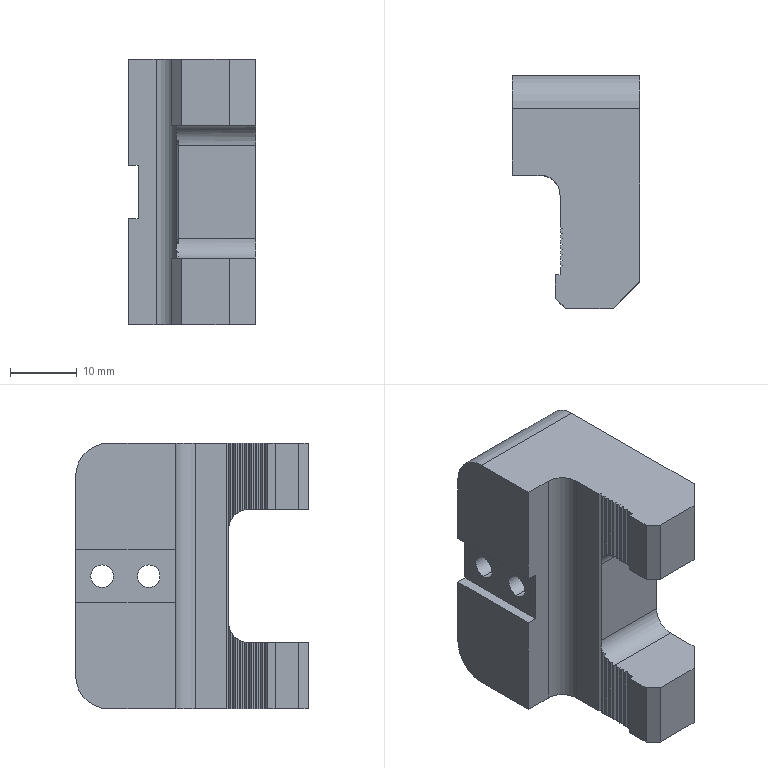Part | STEP file | PN_0053 | 1 solid | 80 faces | box 19.2 x 35 x 39.94 mm | volume 17498 mm3 | plane 71 | cylinder 9 | commonest cylinder face diameters 3.4 x4 6 x3 10 x2